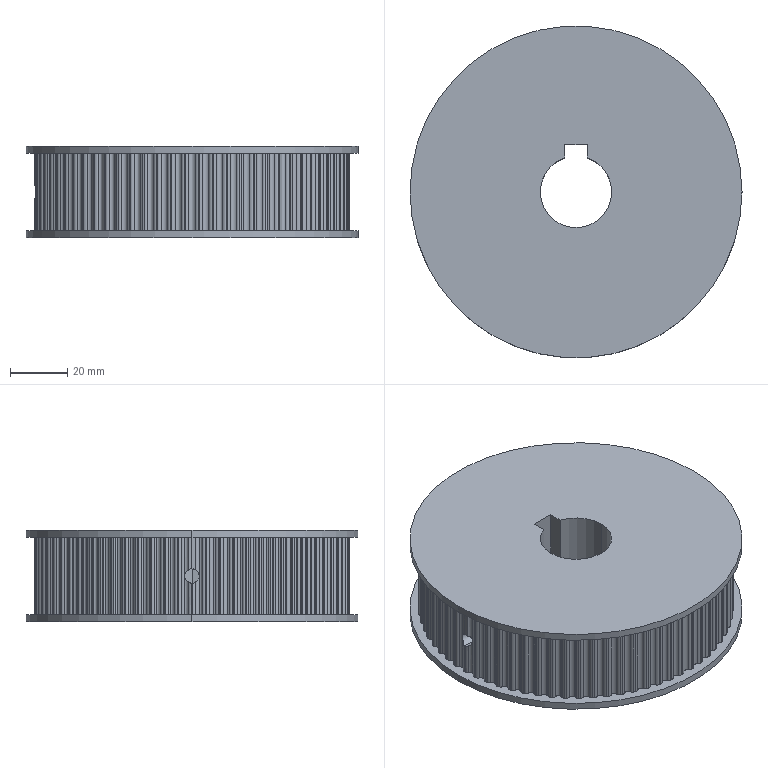Part | 1 solid | 348 faces | box 116 x 116 x 32 mm | volume 285965 mm3 | cylinder 341 | plane 7 | commonest cylinder face diameters 2.5 x257 110 x73 5 x4 116 x4 25 x3